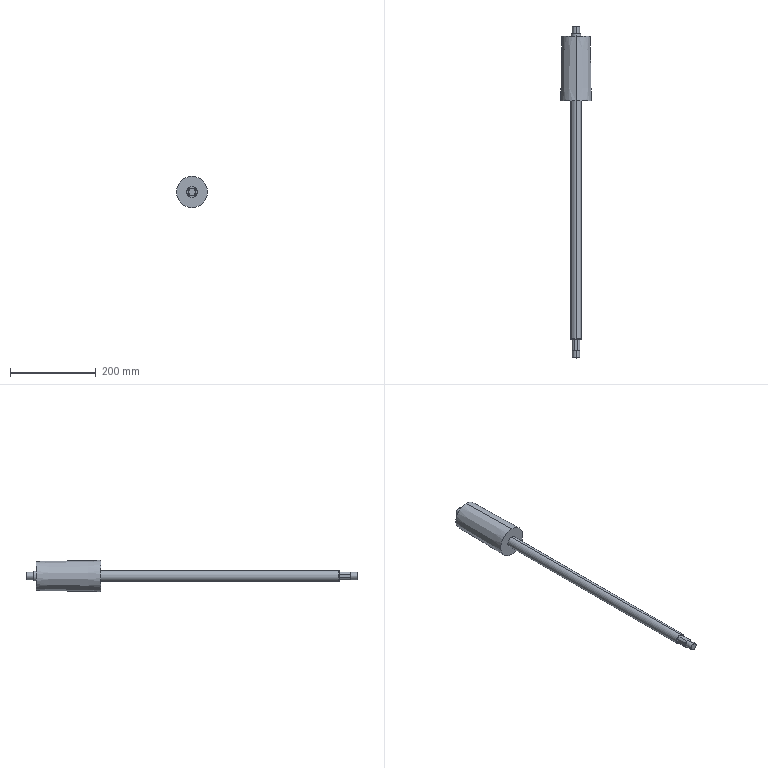Part | STEP file | bevel drive wheel_SUS304 | 1 solid | 33 faces | box 72.6 x 773 x 72.6 mm | volume 867649 mm3 | cylinder 12 | plane 11 | cone 10 | commonest cylinder face diameters 17 x4 20 x4 22 x2 25 x2